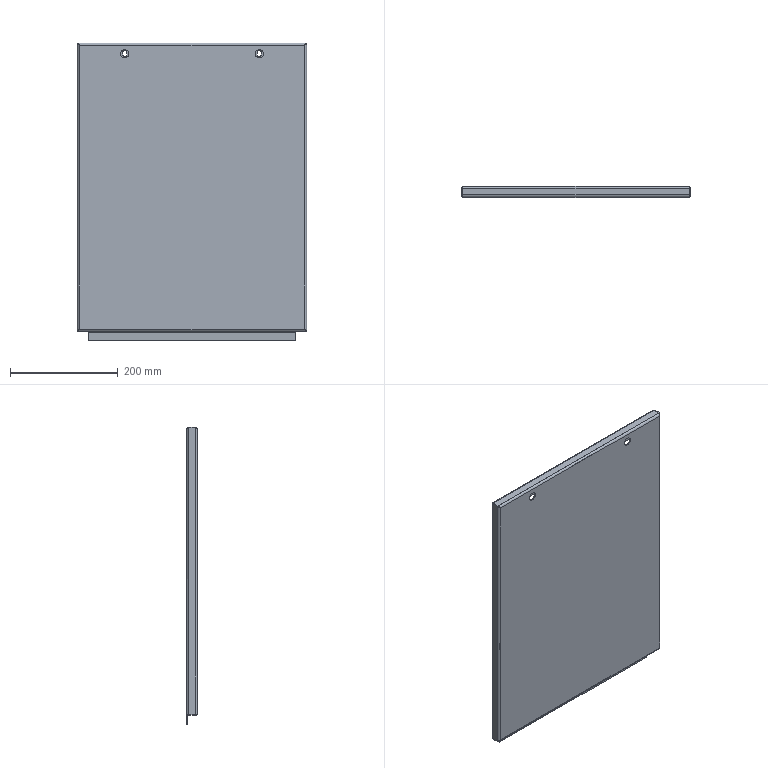Part | NX | features solid 2 | 1 solid | 106 faces | box 426 x 20 x 554 mm | volume 592374 mm3 | plane 70 | cylinder 28 | spline 8 | commonest cylinder face diameters 8 x10 4 x8 7 x6 15 x4